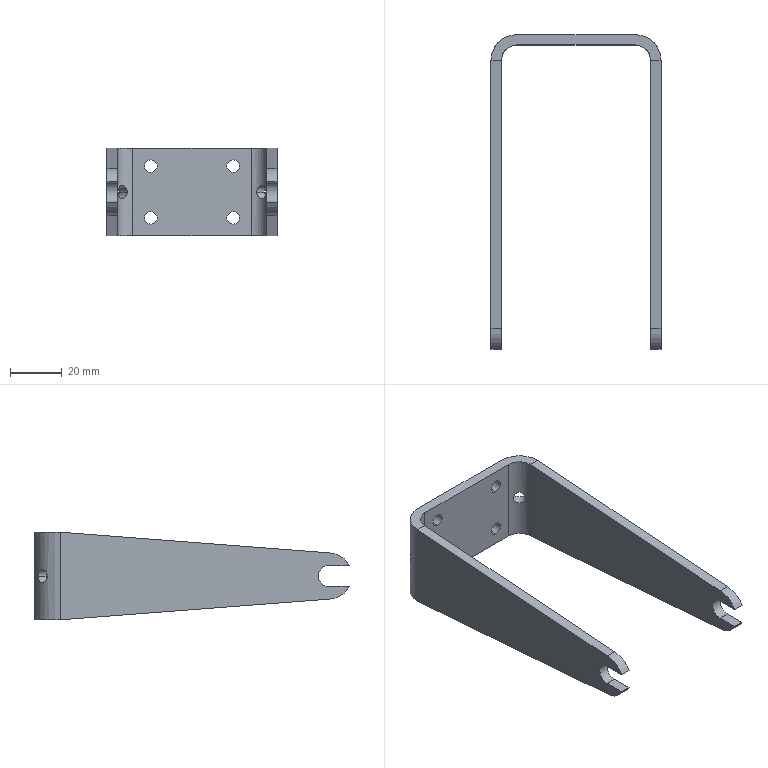Part | SolidWorks | features BaseBody 1 | 1 solid | 38 faces | box 66 x 122.062 x 34 mm | volume 31105 mm3 | cylinder 22 | plane 16 | commonest cylinder face diameters 4.9 x8 5 x4 18 x4 8 x2 12 x2 20 x2
STEP:
#1=CARTESIAN_POINT('',(25.089,57.125,0.));
#2=VERTEX_POINT('',#1);
#3=CARTESIAN_POINT('',(28.625,53.589,0.));
#4=VERTEX_POINT('',#3);
#5=CARTESIAN_POINT('',(25.089,57.125,0.));
#6=CARTESIAN_POINT('',(25.089,57.125,-0.1672));
#7=CARTESIAN_POINT('',(25.106,57.118,-0.3312));
#8=CARTESIAN_POINT('',(25.172,57.093,-0.6531));
#9=CARTESIAN_POINT('',(25.222,57.074,-0.8126));
#10=CARTESIAN_POINT('',(25.348,57.022,-1.114));
#11=CARTESIAN_POINT('',(25.424,56.989,-1.257));
#12=CARTESIAN_POINT('',(25.6,56.908,-1.527));
#13=CARTESIAN_POINT('',(25.698,56.86,-1.653));
#14=CARTESIAN_POINT('',(26.014,56.693,-1.995));
#15=CARTESIAN_POINT('',(26.258,56.548,-2.181));
#16=CARTESIAN_POINT('',(26.628,56.281,-2.369));
#17=CARTESIAN_POINT('',(26.755,56.182,-2.418));
#18=CARTESIAN_POINT('',(27.003,55.972,-2.483));
#19=CARTESIAN_POINT('',(27.123,55.862,-2.5));
#20=CARTESIAN_POINT('',(27.357,55.628,-2.5));
#21=CARTESIAN_POINT('',(27.471,55.505,-2.484));
#22=CARTESIAN_POINT('',(27.68,55.258,-2.419));
#23=CARTESIAN_POINT('',(27.778,55.133,-2.371));
#24=CARTESIAN_POINT('',(27.958,54.882,-2.244));
#25=CARTESIAN_POINT('',(28.039,54.761,-2.167));
#26=CARTESIAN_POINT('',(28.184,54.525,-1.986));
#27=CARTESIAN_POINT('',(28.248,54.41,-1.882));
#28=CARTESIAN_POINT('',(28.36,54.199,-1.654));
#29=CARTESIAN_POINT('',(28.408,54.101,-1.529));
#30=CARTESIAN_POINT('',(28.489,53.926,-1.26));
#31=CARTESIAN_POINT('',(28.522,53.849,-1.115));
#32=CARTESIAN_POINT('',(28.599,53.66,-0.6651));
#33=CARTESIAN_POINT('',(28.625,53.589,-0.3345));
#34=CARTESIAN_POINT('',(28.625,53.589,0.));
#35=B_SPLINE_CURVE_WITH_KNOTS('',3,(#5,#6,#7,#8,#9,#10,#11,#12,#13,#14,#15,#16,#17,#18,#19,#20,#21,#22,#23,#24,#25,#26,#27,#28,#29,#30,#31,#32,#33,#34),.UNSPECIFIED.,.F.,.F.,(4,2,2,2,2,2,2,2,2,2,2,2,2,2,4),(0.,0.0004939,0.0009879,0.001482,0.001976,0.002964,0.003458,0.003952,0.004446,0.004939,0.005433,0.005927,0.006421,0.006915,0.007903),.UNSPECIFIED.);
#36=EDGE_CURVE('',#2,#4,#35,.T.);
#37=ORIENTED_EDGE('',*,*,#36,.T.);
#38=CARTESIAN_POINT('',(31.614,56.579,0.));
#39=VERTEX_POINT('',#38);
#40=CARTESIAN_POINT('',(28.605,53.57,0.));
#41=DIRECTION('',(0.7071,0.7071,0.));
#42=VECTOR('',#41,1000.);
#43=LINE('',#40,#42);
#44=EDGE_CURVE('',#4,#39,#43,.T.);
#45=ORIENTED_EDGE('',*,*,#44,.T.);
#46=CARTESIAN_POINT('',(28.079,60.114,0.));
#47=VERTEX_POINT('',#46);
#48=CARTESIAN_POINT('',(31.614,56.579,0.));
#49=CARTESIAN_POINT('',(31.614,56.579,-0.1658));
#50=CARTESIAN_POINT('',(31.606,56.593,-0.3288));
#51=CARTESIAN_POINT('',(31.572,56.65,-0.6491));
#52=CARTESIAN_POINT('',(31.546,56.693,-0.8082));
#53=CARTESIAN_POINT('',(31.479,56.803,-1.111));
#54=CARTESIAN_POINT('',(31.437,56.869,-1.254));
#55=CARTESIAN_POINT('',(31.336,57.025,-1.525));
#56=CARTESIAN_POINT('',(31.276,57.114,-1.653));
#57=CARTESIAN_POINT('',(31.077,57.401,-1.997));
#58=CARTESIAN_POINT('',(30.909,57.627,-2.183));
#59=CARTESIAN_POINT('',(30.621,57.976,-2.371));
#60=CARTESIAN_POINT('',(30.518,58.096,-2.419));
#61=CARTESIAN_POINT('',(30.301,58.336,-2.484));
#62=CARTESIAN_POINT('',(30.188,58.454,-2.5));
#63=CARTESIAN_POINT('',(29.957,58.685,-2.5));
#64=CARTESIAN_POINT('',(29.836,58.8,-2.484));
#65=CARTESIAN_POINT('',(29.598,59.016,-2.42));
#66=CARTESIAN_POINT('',(29.48,59.118,-2.372));
#67=CARTESIAN_POINT('',(29.127,59.409,-2.184));
#68=CARTESIAN_POINT('',(28.904,59.575,-2.));
#69=CARTESIAN_POINT('',(28.614,59.776,-1.653));
#70=CARTESIAN_POINT('',(28.526,59.835,-1.527));
#71=CARTESIAN_POINT('',(28.371,59.936,-1.257));
#72=CARTESIAN_POINT('',(28.303,59.978,-1.111));
#73=CARTESIAN_POINT('',(28.193,60.046,-0.8094));
#74=CARTESIAN_POINT('',(28.151,60.071,-0.6536));
#75=CARTESIAN_POINT('',(28.094,60.106,-0.3318));
#76=CARTESIAN_POINT('',(28.079,60.114,-0.1658));
#77=CARTESIAN_POINT('',(28.079,60.114,0.));
#78=B_SPLINE_CURVE_WITH_KNOTS('',3,(#48,#49,#50,#51,#52,#53,#54,#55,#56,#57,#58,#59,#60,#61,#62,#63,#64,#65,#66,#67,#68,#69,#70,#71,#72,#73,#74,#75,#76,#77),.UNSPECIFIED.,.F.,.F.,(4,2,2,2,2,2,2,2,2,2,2,2,2,2,4),(0.,0.0004903,0.0009806,0.001471,0.001961,0.002942,0.003432,0.003922,0.004413,0.004903,0.005884,0.006374,0.006864,0.007355,0.007845),.UNSPECIFIED.);
#79=EDGE_CURVE('',#39,#47,#78,.T.);
#80=ORIENTED_EDGE('',*,*,#79,.T.);
#81=CARTESIAN_POINT('',(25.07,57.105,0.));
#82=DIRECTION('',(0.7071,0.7071,0.));
#83=VECTOR('',#82,1000.);
#84=LINE('',#81,#83);
#85=EDGE_CURVE('',#2,#47,#84,.T.);
#86=ORIENTED_EDGE('',*,*,#85,.F.);
#87=EDGE_LOOP('',(#37,#45,#80,#86));
#88=FACE_OUTER_BOUND('',#87,.T.);
#89=CARTESIAN_POINT('',(26.838,55.338,0.));
#90=DIRECTION('',(0.7071,0.7071,0.));
#91=DIRECTION('',(-0.7071,0.7071,0.));
#92=AXIS2_PLACEMENT_3D('',#89,#90,#91);
#93=CYLINDRICAL_SURFACE('',#92,2.5);
#94=ADVANCED_FACE('',(#88),#93,.F.);
#95=CARTESIAN_POINT('',(-16.,57.5,-7.55));
#96=VERTEX_POINT('',#95);
#97=CARTESIAN_POINT('',(-16.,57.5,-12.45));
#98=VERTEX_POINT('',#97);
#99=CARTESIAN_POINT('',(-16.,57.5,-10.));
#100=DIRECTION('',(0.,-1.,0.));
#101=DIRECTION('',(0.,0.,1.));
#102=AXIS2_PLACEMENT_3D('',#99,#100,#101);
#103=CIRCLE('',#102,2.45);
#104=EDGE_CURVE('',#96,#98,#103,.T.);
#105=ORIENTED_EDGE('',*,*,#104,.T.);
#106=CARTESIAN_POINT('',(-16.,61.5,-12.45));
#107=VERTEX_POINT('',#106);
#108=CARTESIAN_POINT('',(-16.,57.5,-12.45));
#109=DIRECTION('',(0.,1.,0.));
#110=VECTOR('',#109,1000.);
#111=LINE('',#108,#110);
#112=EDGE_CURVE('',#98,#107,#111,.T.);
#113=ORIENTED_EDGE('',*,*,#112,.T.);
#114=CARTESIAN_POINT('',(-16.,61.5,-7.55));
#115=VERTEX_POINT('',#114);
#116=CARTESIAN_POINT('',(-16.,61.5,-10.));
#117=DIRECTION('',(0.,1.,0.));
#118=DIRECTION('',(0.,0.,1.));
#119=AXIS2_PLACEMENT_3D('',#116,#117,#118);
#120=CIRCLE('',#119,2.45);
#121=EDGE_CURVE('',#107,#115,#120,.T.);
#122=ORIENTED_EDGE('',*,*,#121,.T.);
#123=CARTESIAN_POINT('',(-16.,57.5,-7.55));
#124=DIRECTION('',(0.,1.,0.));
#125=VECTOR('',#124,1000.);
#126=LINE('',#123,#125);
#127=EDGE_CURVE('',#96,#115,#126,.T.);
#128=ORIENTED_EDGE('',*,*,#127,.F.);
#129=EDGE_LOOP('',(#105,#113,#122,#128));
#130=FACE_OUTER_BOUND('',#129,.T.);
#131=CARTESIAN_POINT('',(-16.,57.5,-10.));
#132=DIRECTION('',(0.,1.,0.));
#133=DIRECTION('',(0.,0.,1.));
#134=AXIS2_PLACEMENT_3D('',#131,#132,#133);
#135=CYLINDRICAL_SURFACE('',#134,2.45);
#136=ADVANCED_FACE('',(#130),#135,.F.);
#137=CARTESIAN_POINT('',(16.,57.5,-7.55));
#138=VERTEX_POINT('',#137);
#139=CARTESIAN_POINT('',(16.,57.5,-12.45));
#140=VERTEX_POINT('',#139);
#141=CARTESIAN_POINT('',(16.,57.5,-10.));
#142=DIRECTION('',(0.,-1.,0.));
#143=DIRECTION('',(0.,0.,1.));
#144=AXIS2_PLACEMENT_3D('',#141,#142,#143);
#145=CIRCLE('',#144,2.45);
#146=EDGE_CURVE('',#138,#140,#145,.T.);
#147=ORIENTED_EDGE('',*,*,#146,.T.);
#148=CARTESIAN_POINT('',(16.,61.5,-12.45));
#149=VERTEX_POINT('',#148);
#150=CARTESIAN_POINT('',(16.,57.5,-12.45));
#151=DIRECTION('',(0.,1.,0.));
#152=VECTOR('',#151,1000.);
#153=LINE('',#150,#152);
#154=EDGE_CURVE('',#140,#149,#153,.T.);
#155=ORIENTED_EDGE('',*,*,#154,.T.);
#156=CARTESIAN_POINT('',(16.,61.5,-7.55));
#157=VERTEX_POINT('',#156);
#158=CARTESIAN_POINT('',(16.,61.5,-10.));
#159=DIRECTION('',(0.,1.,0.));
#160=DIRECTION('',(0.,0.,1.));
#161=AXIS2_PLACEMENT_3D('',#158,#159,#160);
#162=CIRCLE('',#161,2.45);
#163=EDGE_CURVE('',#149,#157,#162,.T.);
#164=ORIENTED_EDGE('',*,*,#163,.T.);
#165=CARTESIAN_POINT('',(16.,57.5,-7.55));
#166=DIRECTION('',(0.,1.,0.));
#167=VECTOR('',#166,1000.);
#168=LINE('',#165,#167);
#169=EDGE_CURVE('',#138,#157,#168,.T.);
#170=ORIENTED_EDGE('',*,*,#169,.F.);
#171=EDGE_LOOP('',(#147,#155,#164,#170));
#172=FACE_OUTER_BOUND('',#171,.T.);
#173=CARTESIAN_POINT('',(16.,57.5,-10.));
#174=DIRECTION('',(0.,1.,0.));
#175=DIRECTION('',(0.,0.,1.));
#176=AXIS2_PLACEMENT_3D('',#173,#174,#175);
#177=CYLINDRICAL_SURFACE('',#176,2.45);
#178=ADVANCED_FACE('',(#172),#177,.F.);
#179=CARTESIAN_POINT('',(-16.,57.5,12.45));
#180=VERTEX_POINT('',#179);
#181=CARTESIAN_POINT('',(-16.,57.5,7.55));
#182=VERTEX_POINT('',#181);
#183=CARTESIAN_POINT('',(-16.,57.5,10.));
#184=DIRECTION('',(0.,-1.,0.));
#185=DIRECTION('',(0.,0.,1.));
#186=AXIS2_PLACEMENT_3D('',#183,#184,#185);
#187=CIRCLE('',#186,2.45);
#188=EDGE_CURVE('',#180,#182,#187,.T.);
#189=ORIENTED_EDGE('',*,*,#188,.T.);
#190=CARTESIAN_POINT('',(-16.,61.5,7.55));
#191=VERTEX_POINT('',#190);
#192=CARTESIAN_POINT('',(-16.,57.5,7.55));
#193=DIRECTION('',(0.,1.,0.));
#194=VECTOR('',#193,1000.);
#195=LINE('',#192,#194);
#196=EDGE_CURVE('',#182,#191,#195,.T.);
#197=ORIENTED_EDGE('',*,*,#196,.T.);
#198=CARTESIAN_POINT('',(-16.,61.5,12.45));
#199=VERTEX_POINT('',#198);
#200=CARTESIAN_POINT('',(-16.,61.5,10.));
#201=DIRECTION('',(0.,1.,0.));
#202=DIRECTION('',(0.,0.,1.));
#203=AXIS2_PLACEMENT_3D('',#200,#201,#202);
#204=CIRCLE('',#203,2.45);
#205=EDGE_CURVE('',#191,#199,#204,.T.);
#206=ORIENTED_EDGE('',*,*,#205,.T.);
#207=CARTESIAN_POINT('',(-16.,57.5,12.45));
#208=DIRECTION('',(0.,1.,0.));
#209=VECTOR('',#208,1000.);
#210=LINE('',#207,#209);
#211=EDGE_CURVE('',#180,#199,#210,.T.);
#212=ORIENTED_EDGE('',*,*,#211,.F.);
#213=EDGE_LOOP('',(#189,#197,#206,#212));
#214=FACE_OUTER_BOUND('',#213,.T.);
#215=CARTESIAN_POINT('',(-16.,57.5,10.));
#216=DIRECTION('',(0.,1.,0.));
#217=DIRECTION('',(0.,0.,1.));
#218=AXIS2_PLACEMENT_3D('',#215,#216,#217);
#219=CYLINDRICAL_SURFACE('',#218,2.45);
#220=ADVANCED_FACE('',(#214),#219,.F.);
#221=CARTESIAN_POINT('',(16.,57.5,12.45));
#222=VERTEX_POINT('',#221);
#223=CARTESIAN_POINT('',(16.,57.5,7.55));
#224=VERTEX_POINT('',#223);
#225=CARTESIAN_POINT('',(16.,57.5,10.));
#226=DIRECTION('',(0.,-1.,0.));
#227=DIRECTION('',(0.,0.,1.));
#228=AXIS2_PLACEMENT_3D('',#225,#226,#227);
#229=CIRCLE('',#228,2.45);
#230=EDGE_CURVE('',#222,#224,#229,.T.);
#231=ORIENTED_EDGE('',*,*,#230,.T.);
#232=CARTESIAN_POINT('',(16.,61.5,7.55));
#233=VERTEX_POINT('',#232);
#234=CARTESIAN_POINT('',(16.,57.5,7.55));
#235=DIRECTION('',(0.,1.,0.));
#236=VECTOR('',#235,1000.);
#237=LINE('',#234,#236);
#238=EDGE_CURVE('',#224,#233,#237,.T.);
#239=ORIENTED_EDGE('',*,*,#238,.T.);
#240=CARTESIAN_POINT('',(16.,61.5,12.45));
#241=VERTEX_POINT('',#240);
#242=CARTESIAN_POINT('',(16.,61.5,10.));
#243=DIRECTION('',(0.,1.,0.));
#244=DIRECTION('',(0.,0.,1.));
#245=AXIS2_PLACEMENT_3D('',#242,#243,#244);
#246=CIRCLE('',#245,2.45);
#247=EDGE_CURVE('',#233,#241,#246,.T.);
#248=ORIENTED_EDGE('',*,*,#247,.T.);
#249=CARTESIAN_POINT('',(16.,57.5,12.45));
#250=DIRECTION('',(0.,1.,0.));
#251=VECTOR('',#250,1000.);
#252=LINE('',#249,#251);
#253=EDGE_CURVE('',#222,#241,#252,.T.);
#254=ORIENTED_EDGE('',*,*,#253,.F.);
#255=EDGE_LOOP('',(#231,#239,#248,#254));
#256=FACE_OUTER_BOUND('',#255,.T.);
#257=CARTESIAN_POINT('',(16.,57.5,10.));
#258=DIRECTION('',(0.,1.,0.));
#259=DIRECTION('',(0.,0.,1.));
#260=AXIS2_PLACEMENT_3D('',#257,#258,#259);
#261=CYLINDRICAL_SURFACE('',#260,2.45);
#262=ADVANCED_FACE('',(#256),#261,.F.);
#263=CARTESIAN_POINT('',(-25.089,57.125,0.));
#264=VERTEX_POINT('',#263);
#265=CARTESIAN_POINT('',(-28.625,53.589,0.));
#266=VERTEX_POINT('',#265);
#267=CARTESIAN_POINT('',(-25.089,57.125,0.));
#268=CARTESIAN_POINT('',(-25.089,57.125,-0.1672));
#269=CARTESIAN_POINT('',(-25.106,57.118,-0.3312));
#270=CARTESIAN_POINT('',(-25.172,57.093,-0.6531));
#271=CARTESIAN_POINT('',(-25.222,57.074,-0.8126));
#272=CARTESIAN_POINT('',(-25.348,57.022,-1.114));
#273=CARTESIAN_POINT('',(-25.424,56.989,-1.257));
#274=CARTESIAN_POINT('',(-25.6,56.908,-1.527));
#275=CARTESIAN_POINT('',(-25.698,56.86,-1.653));
#276=CARTESIAN_POINT('',(-26.014,56.693,-1.995));
#277=CARTESIAN_POINT('',(-26.258,56.548,-2.181));
#278=CARTESIAN_POINT('',(-26.628,56.281,-2.369));
#279=CARTESIAN_POINT('',(-26.755,56.182,-2.418));
#280=CARTESIAN_POINT('',(-27.003,55.972,-2.483));
#281=CARTESIAN_POINT('',(-27.123,55.862,-2.5));
#282=CARTESIAN_POINT('',(-27.357,55.628,-2.5));
#283=CARTESIAN_POINT('',(-27.471,55.505,-2.484));
#284=CARTESIAN_POINT('',(-27.68,55.258,-2.419));
#285=CARTESIAN_POINT('',(-27.778,55.133,-2.371));
#286=CARTESIAN_POINT('',(-27.958,54.882,-2.244));
#287=CARTESIAN_POINT('',(-28.039,54.761,-2.167));
#288=CARTESIAN_POINT('',(-28.184,54.525,-1.986));
#289=CARTESIAN_POINT('',(-28.248,54.41,-1.882));
#290=CARTESIAN_POINT('',(-28.36,54.199,-1.654));
#291=CARTESIAN_POINT('',(-28.408,54.101,-1.529));
#292=CARTESIAN_POINT('',(-28.489,53.926,-1.26));
#293=CARTESIAN_POINT('',(-28.522,53.849,-1.115));
#294=CARTESIAN_POINT('',(-28.599,53.66,-0.6651));
#295=CARTESIAN_POINT('',(-28.625,53.589,-0.3343));
#296=CARTESIAN_POINT('',(-28.625,53.589,0.));
#297=B_SPLINE_CURVE_WITH_KNOTS('',3,(#267,#268,#269,#270,#271,#272,#273,#274,#275,#276,#277,#278,#279,#280,#281,#282,#283,#284,#285,#286,#287,#288,#289,#290,#291,#292,#293,#294,#295,#296),.UNSPECIFIED.,.F.,.F.,(4,2,2,2,2,2,2,2,2,2,2,2,2,2,4),(0.007903,0.008397,0.008891,0.009385,0.009878,0.01087,0.01136,0.01185,0.01235,0.01284,0.01334,0.01383,0.01432,0.01482,0.0158),.UNSPECIFIED.);
#298=EDGE_CURVE('',#264,#266,#297,.T.);
#299=ORIENTED_EDGE('',*,*,#298,.F.);
#300=CARTESIAN_POINT('',(-28.079,60.114,0.));
#301=VERTEX_POINT('',#300);
#302=CARTESIAN_POINT('',(-25.07,57.105,0.));
#303=DIRECTION('',(-0.7071,0.7071,0.));
#304=VECTOR('',#303,1000.);
#305=LINE('',#302,#304);
#306=EDGE_CURVE('',#264,#301,#305,.T.);
#307=ORIENTED_EDGE('',*,*,#306,.T.);
#308=CARTESIAN_POINT('',(-31.614,56.579,0.));
#309=VERTEX_POINT('',#308);
#310=CARTESIAN_POINT('',(-28.079,60.114,0.));
#311=CARTESIAN_POINT('',(-28.079,60.114,-0.1658));
#312=CARTESIAN_POINT('',(-28.093,60.106,-0.3288));
#313=CARTESIAN_POINT('',(-28.15,60.072,-0.6491));
#314=CARTESIAN_POINT('',(-28.193,60.046,-0.8082));
#315=CARTESIAN_POINT('',(-28.303,59.979,-1.111));
#316=CARTESIAN_POINT('',(-28.369,59.937,-1.254));
#317=CARTESIAN_POINT('',(-28.525,59.836,-1.525));
#318=CARTESIAN_POINT('',(-28.614,59.776,-1.653));
#319=CARTESIAN_POINT('',(-28.901,59.577,-1.997));
#320=CARTESIAN_POINT('',(-29.127,59.409,-2.183));
#321=CARTESIAN_POINT('',(-29.476,59.121,-2.371));
#322=CARTESIAN_POINT('',(-29.596,59.018,-2.419));
#323=CARTESIAN_POINT('',(-29.836,58.801,-2.484));
#324=CARTESIAN_POINT('',(-29.954,58.688,-2.5));
#325=CARTESIAN_POINT('',(-30.185,58.457,-2.5));
#326=CARTESIAN_POINT('',(-30.3,58.336,-2.484));
#327=CARTESIAN_POINT('',(-30.516,58.098,-2.42));
#328=CARTESIAN_POINT('',(-30.618,57.98,-2.372));
#329=CARTESIAN_POINT('',(-30.909,57.627,-2.184));
#330=CARTESIAN_POINT('',(-31.075,57.404,-2.));
#331=CARTESIAN_POINT('',(-31.276,57.114,-1.653));
#332=CARTESIAN_POINT('',(-31.335,57.026,-1.527));
#333=CARTESIAN_POINT('',(-31.436,56.871,-1.257));
#334=CARTESIAN_POINT('',(-31.478,56.803,-1.111));
#335=CARTESIAN_POINT('',(-31.546,56.693,-0.8094));
#336=CARTESIAN_POINT('',(-31.571,56.651,-0.6536));
#337=CARTESIAN_POINT('',(-31.606,56.594,-0.3318));
#338=CARTESIAN_POINT('',(-31.614,56.579,-0.1658));
#339=CARTESIAN_POINT('',(-31.614,56.579,0.));
#340=B_SPLINE_CURVE_WITH_KNOTS('',3,(#310,#311,#312,#313,#314,#315,#316,#317,#318,#319,#320,#321,#322,#323,#324,#325,#326,#327,#328,#329,#330,#331,#332,#333,#334,#335,#336,#337,#338,#339),.UNSPECIFIED.,.F.,.F.,(4,2,2,2,2,2,2,2,2,2,2,2,2,2,4),(0.007845,0.008335,0.008825,0.009316,0.009806,0.01079,0.01128,0.01177,0.01226,0.01275,0.01373,0.01422,0.01471,0.0152,0.01569),.UNSPECIFIED.);
#341=EDGE_CURVE('',#301,#309,#340,.T.);
#342=ORIENTED_EDGE('',*,*,#341,.T.);
#343=CARTESIAN_POINT('',(-28.605,53.57,0.));
#344=DIRECTION('',(-0.7071,0.7071,0.));
#345=VECTOR('',#344,1000.);
#346=LINE('',#343,#345);
#347=EDGE_CURVE('',#266,#309,#346,.T.);
#348=ORIENTED_EDGE('',*,*,#347,.F.);
#349=EDGE_LOOP('',(#299,#307,#342,#348));
#350=FACE_OUTER_BOUND('',#349,.T.);
#351=CARTESIAN_POINT('',(-26.838,55.338,0.));
#352=DIRECTION('',(-0.7071,0.7071,0.));
#353=DIRECTION('',(-0.7071,-0.7071,0.));
#354=AXIS2_PLACEMENT_3D('',#351,#352,#353);
#355=CYLINDRICAL_SURFACE('',#354,2.5);
#356=ADVANCED_FACE('',(#350),#355,.F.);
#357=ORIENTED_EDGE('',*,*,#44,.F.);
#358=CARTESIAN_POINT('',(28.625,53.589,0.));
#359=CARTESIAN_POINT('',(28.625,53.589,0.1672));
#360=CARTESIAN_POINT('',(28.618,53.606,0.3312));
#361=CARTESIAN_POINT('',(28.593,53.672,0.6531));
#362=CARTESIAN_POINT('',(28.574,53.722,0.8126));
#363=CARTESIAN_POINT('',(28.522,53.848,1.114));
#364=CARTESIAN_POINT('',(28.489,53.924,1.257));
#365=CARTESIAN_POINT('',(28.408,54.1,1.527));
#366=CARTESIAN_POINT('',(28.36,54.198,1.653));
#367=CARTESIAN_POINT('',(28.193,54.514,1.995));
#368=CARTESIAN_POINT('',(28.048,54.758,2.181));
#369=CARTESIAN_POINT('',(27.781,55.128,2.369));
#370=CARTESIAN_POINT('',(27.682,55.255,2.418));
#371=CARTESIAN_POINT('',(27.472,55.503,2.483));
#372=CARTESIAN_POINT('',(27.362,55.623,2.5));
#373=CARTESIAN_POINT('',(27.128,55.857,2.5));
#374=CARTESIAN_POINT('',(27.005,55.971,2.484));
#375=CARTESIAN_POINT('',(26.758,56.18,2.419));
#376=CARTESIAN_POINT('',(26.633,56.278,2.371));
#377=CARTESIAN_POINT('',(26.382,56.458,2.244));
#378=CARTESIAN_POINT('',(26.261,56.539,2.167));
#379=CARTESIAN_POINT('',(26.025,56.684,1.986));
#380=CARTESIAN_POINT('',(25.91,56.748,1.882));
#381=CARTESIAN_POINT('',(25.699,56.86,1.654));
#382=CARTESIAN_POINT('',(25.601,56.908,1.529));
#383=CARTESIAN_POINT('',(25.426,56.989,1.26));
#384=CARTESIAN_POINT('',(25.349,57.022,1.115));
#385=CARTESIAN_POINT('',(25.16,57.099,0.6651));
#386=CARTESIAN_POINT('',(25.089,57.125,0.3343));
#387=CARTESIAN_POINT('',(25.089,57.125,0.));
#388=B_SPLINE_CURVE_WITH_KNOTS('',3,(#358,#359,#360,#361,#362,#363,#364,#365,#366,#367,#368,#369,#370,#371,#372,#373,#374,#375,#376,#377,#378,#379,#380,#381,#382,#383,#384,#385,#386,#387),.UNSPECIFIED.,.F.,.F.,(4,2,2,2,2,2,2,2,2,2,2,2,2,2,4),(0.007903,0.008397,0.008891,0.009385,0.009878,0.01087,0.01136,0.01185,0.01235,0.01284,0.01334,0.01383,0.01432,0.01482,0.0158),.UNSPECIFIED.);
#389=EDGE_CURVE('',#4,#2,#388,.T.);
#390=ORIENTED_EDGE('',*,*,#389,.T.);
#391=ORIENTED_EDGE('',*,*,#85,.T.);
#392=CARTESIAN_POINT('',(28.079,60.114,0.));
#393=CARTESIAN_POINT('',(28.079,60.114,0.1658));
#394=CARTESIAN_POINT('',(28.093,60.106,0.3288));
#395=CARTESIAN_POINT('',(28.15,60.072,0.6491));
#396=CARTESIAN_POINT('',(28.193,60.046,0.8082));
#397=CARTESIAN_POINT('',(28.303,59.979,1.111));
#398=CARTESIAN_POINT('',(28.369,59.937,1.254));
#399=CARTESIAN_POINT('',(28.525,59.836,1.525));
#400=CARTESIAN_POINT('',(28.614,59.776,1.653));
#401=CARTESIAN_POINT('',(28.901,59.577,1.997));
#402=CARTESIAN_POINT('',(29.127,59.409,2.183));
#403=CARTESIAN_POINT('',(29.476,59.121,2.371));
#404=CARTESIAN_POINT('',(29.596,59.018,2.419));
#405=CARTESIAN_POINT('',(29.836,58.801,2.484));
#406=CARTESIAN_POINT('',(29.954,58.688,2.5));
#407=CARTESIAN_POINT('',(30.185,58.457,2.5));
#408=CARTESIAN_POINT('',(30.3,58.336,2.484));
#409=CARTESIAN_POINT('',(30.516,58.098,2.42));
#410=CARTESIAN_POINT('',(30.618,57.98,2.372));
#411=CARTESIAN_POINT('',(30.909,57.627,2.184));
#412=CARTESIAN_POINT('',(31.075,57.404,2.));
#413=CARTESIAN_POINT('',(31.276,57.114,1.653));
#414=CARTESIAN_POINT('',(31.335,57.026,1.527));
#415=CARTESIAN_POINT('',(31.436,56.871,1.257));
#416=CARTESIAN_POINT('',(31.478,56.803,1.111));
#417=CARTESIAN_POINT('',(31.546,56.693,0.8094));
#418=CARTESIAN_POINT('',(31.571,56.651,0.6536));
#419=CARTESIAN_POINT('',(31.606,56.594,0.3318));
#420=CARTESIAN_POINT('',(31.614,56.579,0.1658));
#421=CARTESIAN_POINT('',(31.614,56.579,0.));
#422=B_SPLINE_CURVE_WITH_KNOTS('',3,(#392,#393,#394,#395,#396,#397,#398,#399,#400,#401,#402,#403,#404,#405,#406,#407,#408,#409,#410,#411,#412,#413,#414,#415,#416,#417,#418,#419,#420,#421),.UNSPECIFIED.,.F.,.F.,(4,2,2,2,2,2,2,2,2,2,2,2,2,2,4),(0.007845,0.008335,0.008825,0.009316,0.009806,0.01079,0.01128,0.01177,0.01226,0.01275,0.01373,0.01422,0.01471,0.0152,0.01569),.UNSPECIFIED.);
#423=EDGE_CURVE('',#47,#39,#422,.T.);
#424=ORIENTED_EDGE('',*,*,#423,.T.);
#425=EDGE_LOOP('',(#357,#390,#391,#424));
#426=FACE_OUTER_BOUND('',#425,.T.);
#427=CARTESIAN_POINT('',(26.838,55.338,0.));
#428=DIRECTION('',(0.7071,0.7071,0.));
#429=DIRECTION('',(-0.7071,0.7071,0.));
#430=AXIS2_PLACEMENT_3D('',#427,#428,#429);
#431=CYLINDRICAL_SURFACE('',#430,2.5);
#432=ADVANCED_FACE('',(#426),#431,.F.);
#433=CARTESIAN_POINT('',(23.,61.5,17.));
#434=VERTEX_POINT('',#433);
#435=CARTESIAN_POINT('',(23.,61.5,-17.));
#436=VERTEX_POINT('',#435);
#437=CARTESIAN_POINT('',(23.,61.5,0.));
#438=DIRECTION('',(0.,0.,-1.));
#439=VECTOR('',#438,1000.);
#440=LINE('',#437,#439);
#441=EDGE_CURVE('',#434,#436,#440,.T.);
#442=ORIENTED_EDGE('',*,*,#441,.F.);
#443=CARTESIAN_POINT('',(33.,51.5,17.));
#444=VERTEX_POINT('',#443);
#445=CARTESIAN_POINT('',(23.,51.5,17.));
#446=DIRECTION('',(0.,0.,1.));
#447=DIRECTION('',(-1.,0.,0.));
#448=AXIS2_PLACEMENT_3D('',#445,#446,#447);
#449=CIRCLE('',#448,10.);
#450=EDGE_CURVE('',#444,#434,#449,.T.);
#451=ORIENTED_EDGE('',*,*,#450,.F.);
#452=CARTESIAN_POINT('',(33.,51.5,-17.));
#453=VERTEX_POINT('',#452);
#454=CARTESIAN_POINT('',(33.,51.5,0.));
#455=DIRECTION('',(0.,0.,1.));
#456=VECTOR('',#455,1000.);
#457=LINE('',#454,#456);
#458=EDGE_CURVE('',#453,#444,#457,.T.);
#459=ORIENTED_EDGE('',*,*,#458,.F.);
#460=CARTESIAN_POINT('',(23.,51.5,-17.));
#461=DIRECTION('',(0.,0.,-1.));
#462=DIRECTION('',(-1.,0.,0.));
#463=AXIS2_PLACEMENT_3D('',#460,#461,#462);
#464=CIRCLE('',#463,10.);
#465=EDGE_CURVE('',#436,#453,#464,.T.);
#466=ORIENTED_EDGE('',*,*,#465,.F.);
#467=EDGE_LOOP('',(#442,#451,#459,#466));
#468=FACE_OUTER_BOUND('',#467,.T.);
#469=ORIENTED_EDGE('',*,*,#423,.F.);
#470=ORIENTED_EDGE('',*,*,#79,.F.);
#471=EDGE_LOOP('',(#469,#470));
#472=FACE_BOUND('',#471,.T.);
#473=CARTESIAN_POINT('',(23.,51.5,17.));
#474=DIRECTION('',(0.,0.,-1.));
#475=DIRECTION('',(-1.,0.,0.));
#476=AXIS2_PLACEMENT_3D('',#473,#474,#475);
#477=CYLINDRICAL_SURFACE('',#476,10.);
#478=ADVANCED_FACE('',(#468,#472),#477,.T.);
#479=CARTESIAN_POINT('',(29.,51.5,17.));
#480=VERTEX_POINT('',#479);
#481=CARTESIAN_POINT('',(23.,57.5,17.));
#482=VERTEX_POINT('',#481);
#483=CARTESIAN_POINT('',(23.,51.5,17.));
#484=DIRECTION('',(0.,0.,1.));
#485=DIRECTION('',(-1.,0.,0.));
#486=AXIS2_PLACEMENT_3D('',#483,#484,#485);
#487=CIRCLE('',#486,6.);
#488=EDGE_CURVE('',#480,#482,#487,.T.);
#489=ORIENTED_EDGE('',*,*,#488,.T.);
#490=CARTESIAN_POINT('',(23.,57.5,-17.));
#491=VERTEX_POINT('',#490);
#492=CARTESIAN_POINT('',(23.,57.5,0.));
#493=DIRECTION('',(0.,0.,-1.));
#494=VECTOR('',#493,1000.);
#495=LINE('',#492,#494);
#496=EDGE_CURVE('',#482,#491,#495,.T.);
#497=ORIENTED_EDGE('',*,*,#496,.T.);
#498=CARTESIAN_POINT('',(29.,51.5,-17.));
#499=VERTEX_POINT('',#498);
#500=CARTESIAN_POINT('',(23.,51.5,-17.));
#501=DIRECTION('',(0.,0.,-1.));
#502=DIRECTION('',(-1.,0.,0.));
#503=AXIS2_PLACEMENT_3D('',#500,#501,#502);
#504=CIRCLE('',#503,6.);
#505=EDGE_CURVE('',#491,#499,#504,.T.);
#506=ORIENTED_EDGE('',*,*,#505,.T.);
#507=CARTESIAN_POINT('',(29.,51.5,0.));
#508=DIRECTION('',(0.,0.,1.));
#509=VECTOR('',#508,1000.);
#510=LINE('',#507,#509);
#511=EDGE_CURVE('',#499,#480,#510,.T.);
#512=ORIENTED_EDGE('',*,*,#511,.T.);
#513=EDGE_LOOP('',(#489,#497,#506,#512));
#514=FACE_OUTER_BOUND('',#513,.T.);
#515=ORIENTED_EDGE('',*,*,#36,.F.);
#516=ORIENTED_EDGE('',*,*,#389,.F.);
#517=EDGE_LOOP('',(#515,#516));
#518=FACE_BOUND('',#517,.T.);
#519=CARTESIAN_POINT('',(23.,51.5,17.));
#520=DIRECTION('',(0.,0.,-1.));
#521=DIRECTION('',(-1.,0.,0.));
#522=AXIS2_PLACEMENT_3D('',#519,#520,#521);
#523=CYLINDRICAL_SURFACE('',#522,6.);
#524=ADVANCED_FACE('',(#514,#518),#523,.F.);
#525=CARTESIAN_POINT('',(0.,51.5,-17.));
#526=DIRECTION('',(1.,0.,0.));
#527=VECTOR('',#526,1000.);
#528=LINE('',#525,#527);
#529=EDGE_CURVE('',#499,#453,#528,.T.);
#530=ORIENTED_EDGE('',*,*,#529,.F.);
#531=ORIENTED_EDGE('',*,*,#505,.F.);
#532=CARTESIAN_POINT('',(-23.,57.5,-17.));
#533=VERTEX_POINT('',#532);
#534=CARTESIAN_POINT('',(0.,57.5,-17.));
#535=DIRECTION('',(1.,0.,0.));
#536=VECTOR('',#535,1000.);
#537=LINE('',#534,#536);
#538=EDGE_CURVE('',#533,#491,#537,.T.);
#539=ORIENTED_EDGE('',*,*,#538,.F.);
#540=CARTESIAN_POINT('',(-29.,51.5,-17.));
#541=VERTEX_POINT('',#540);
#542=CARTESIAN_POINT('',(-23.,51.5,-17.));
#543=DIRECTION('',(0.,0.,-1.));
#544=DIRECTION('',(-1.,0.,0.));
#545=AXIS2_PLACEMENT_3D('',#542,#543,#544);
#546=CIRCLE('',#545,6.);
#547=EDGE_CURVE('',#541,#533,#546,.T.);
#548=ORIENTED_EDGE('',*,*,#547,.F.);
#549=CARTESIAN_POINT('',(-33.,51.5,-17.));
#550=VERTEX_POINT('',#549);
#551=CARTESIAN_POINT('',(0.,51.5,-17.));
#552=DIRECTION('',(1.,0.,0.));
#553=VECTOR('',#552,1000.);
#554=LINE('',#551,#553);
#555=EDGE_CURVE('',#550,#541,#554,.T.);
#556=ORIENTED_EDGE('',*,*,#555,.F.);
#557=CARTESIAN_POINT('',(-23.,61.5,-17.));
#558=VERTEX_POINT('',#557);
#559=CARTESIAN_POINT('',(-23.,51.5,-17.));
#560=DIRECTION('',(0.,0.,1.));
#561=DIRECTION('',(-1.,0.,0.));
#562=AXIS2_PLACEMENT_3D('',#559,#560,#561);
#563=CIRCLE('',#562,10.);
#564=EDGE_CURVE('',#558,#550,#563,.T.);
#565=ORIENTED_EDGE('',*,*,#564,.F.);
#566=CARTESIAN_POINT('',(0.,61.5,-17.));
#567=DIRECTION('',(-1.,0.,0.));
#568=VECTOR('',#567,1000.);
#569=LINE('',#566,#568);
#570=EDGE_CURVE('',#436,#558,#569,.T.);
#571=ORIENTED_EDGE('',*,*,#570,.F.);
#572=ORIENTED_EDGE('',*,*,#465,.T.);
#573=EDGE_LOOP('',(#530,#531,#539,#548,#556,#565,#571,#572));
#574=FACE_OUTER_BOUND('',#573,.T.);
#575=CARTESIAN_POINT('',(-33.396,51.5,-17.));
#576=DIRECTION('',(0.,0.,1.));
#577=DIRECTION('',(1.,0.,0.));
#578=AXIS2_PLACEMENT_3D('',#575,#576,#577);
#579=PLANE('',#578);
#580=ADVANCED_FACE('',(#574),#579,.F.);
#581=CARTESIAN_POINT('',(-16.,61.5,-10.));
#582=DIRECTION('',(0.,1.,0.));
#583=DIRECTION('',(0.,0.,1.));
#584=AXIS2_PLACEMENT_3D('',#581,#582,#583);
#585=CIRCLE('',#584,2.45);
#586=EDGE_CURVE('',#115,#107,#585,.T.);
#587=ORIENTED_EDGE('',*,*,#586,.F.);
#588=ORIENTED_EDGE('',*,*,#121,.F.);
#589=EDGE_LOOP('',(#587,#588));
#590=FACE_BOUND('',#589,.T.);
#591=CARTESIAN_POINT('',(16.,61.5,-10.));
#592=DIRECTION('',(0.,1.,0.));
#593=DIRECTION('',(0.,0.,1.));
#594=AXIS2_PLACEMENT_3D('',#591,#592,#593);
#595=CIRCLE('',#594,2.45);
#596=EDGE_CURVE('',#157,#149,#595,.T.);
#597=ORIENTED_EDGE('',*,*,#596,.F.);
#598=ORIENTED_EDGE('',*,*,#163,.F.);
#599=EDGE_LOOP('',(#597,#598));
#600=FACE_BOUND('',#599,.T.);
#601=CARTESIAN_POINT('',(-16.,61.5,10.));
#602=DIRECTION('',(0.,1.,0.));
#603=DIRECTION('',(0.,0.,1.));
#604=AXIS2_PLACEMENT_3D('',#601,#602,#603);
#605=CIRCLE('',#604,2.45);
#606=EDGE_CURVE('',#199,#191,#605,.T.);
#607=ORIENTED_EDGE('',*,*,#606,.F.);
#608=ORIENTED_EDGE('',*,*,#205,.F.);
#609=EDGE_LOOP('',(#607,#608));
#610=FACE_BOUND('',#609,.T.);
#611=CARTESIAN_POINT('',(16.,61.5,10.));
#612=DIRECTION('',(0.,1.,0.));
#613=DIRECTION('',(0.,0.,1.));
#614=AXIS2_PLACEMENT_3D('',#611,#612,#613);
#615=CIRCLE('',#614,2.45);
#616=EDGE_CURVE('',#241,#233,#615,.T.);
#617=ORIENTED_EDGE('',*,*,#616,.F.);
#618=ORIENTED_EDGE('',*,*,#247,.F.);
#619=EDGE_LOOP('',(#617,#618));
#620=FACE_BOUND('',#619,.T.);
#621=CARTESIAN_POINT('',(-23.,61.5,17.));
#622=VERTEX_POINT('',#621);
#623=CARTESIAN_POINT('',(-23.,61.5,0.));
#624=DIRECTION('',(0.,0.,-1.));
#625=VECTOR('',#624,1000.);
#626=LINE('',#623,#625);
#627=EDGE_CURVE('',#622,#558,#626,.T.);
#628=ORIENTED_EDGE('',*,*,#627,.F.);
#629=CARTESIAN_POINT('',(0.,61.5,17.));
#630=DIRECTION('',(-1.,0.,0.));
#631=VECTOR('',#630,1000.);
#632=LINE('',#629,#631);
#633=EDGE_CURVE('',#434,#622,#632,.T.);
#634=ORIENTED_EDGE('',*,*,#633,.F.);
#635=ORIENTED_EDGE('',*,*,#441,.T.);
#636=ORIENTED_EDGE('',*,*,#570,.T.);
#637=EDGE_LOOP('',(#628,#634,#635,#636));
#638=FACE_OUTER_BOUND('',#637,.T.);
#639=CARTESIAN_POINT('',(-23.,61.5,-17.));
#640=DIRECTION('',(0.,-1.,0.));
#641=DIRECTION('',(1.,0.,0.));
#642=AXIS2_PLACEMENT_3D('',#639,#640,#641);
#643=PLANE('',#642);
#644=ADVANCED_FACE('',(#590,#600,#610,#620,#638),#643,.F.);
#645=CARTESIAN_POINT('',(-23.,57.5,17.));
#646=VERTEX_POINT('',#645);
#647=CARTESIAN_POINT('',(0.,57.5,17.));
#648=DIRECTION('',(1.,0.,0.));
#649=VECTOR('',#648,1000.);
#650=LINE('',#647,#649);
#651=EDGE_CURVE('',#646,#482,#650,.T.);
#652=ORIENTED_EDGE('',*,*,#651,.T.);
#653=ORIENTED_EDGE('',*,*,#488,.F.);
#654=CARTESIAN_POINT('',(0.,51.5,17.));
#655=DIRECTION('',(1.,0.,0.));
#656=VECTOR('',#655,1000.);
#657=LINE('',#654,#656);
#658=EDGE_CURVE('',#480,#444,#657,.T.);
#659=ORIENTED_EDGE('',*,*,#658,.T.);
#660=ORIENTED_EDGE('',*,*,#450,.T.);
#661=ORIENTED_EDGE('',*,*,#633,.T.);
#662=CARTESIAN_POINT('',(-33.,51.5,17.));
#663=VERTEX_POINT('',#662);
#664=CARTESIAN_POINT('',(-23.,51.5,17.));
#665=DIRECTION('',(0.,0.,1.));
#666=DIRECTION('',(-1.,0.,0.));
#667=AXIS2_PLACEMENT_3D('',#664,#665,#666);
#668=CIRCLE('',#667,10.);
#669=EDGE_CURVE('',#622,#663,#668,.T.);
#670=ORIENTED_EDGE('',*,*,#669,.T.);
#671=CARTESIAN_POINT('',(-29.,51.5,17.));
#672=VERTEX_POINT('',#671);
#673=CARTESIAN_POINT('',(0.,51.5,17.));
#674=DIRECTION('',(1.,0.,0.));
#675=VECTOR('',#674,1000.);
#676=LINE('',#673,#675);
#677=EDGE_CURVE('',#663,#672,#676,.T.);
#678=ORIENTED_EDGE('',*,*,#677,.T.);
#679=CARTESIAN_POINT('',(-23.,51.5,17.));
#680=DIRECTION('',(0.,0.,-1.));
#681=DIRECTION('',(-1.,0.,0.));
#682=AXIS2_PLACEMENT_3D('',#679,#680,#681);
#683=CIRCLE('',#682,6.);
#684=EDGE_CURVE('',#672,#646,#683,.T.);
#685=ORIENTED_EDGE('',*,*,#684,.T.);
#686=EDGE_LOOP('',(#652,#653,#659,#660,#661,#670,#678,#685));
#687=FACE_OUTER_BOUND('',#686,.T.);
#688=CARTESIAN_POINT('',(-33.396,51.5,17.));
#689=DIRECTION('',(0.,0.,1.));
#690=DIRECTION('',(1.,0.,0.));
#691=AXIS2_PLACEMENT_3D('',#688,#689,#690);
#692=PLANE('',#691);
#693=ADVANCED_FACE('',(#687),#692,.T.);
#694=CARTESIAN_POINT('',(33.,-52.5,9.));
#695=VERTEX_POINT('',#694);
#696=CARTESIAN_POINT('',(33.,-52.5,9.));
#697=DIRECTION('',(0.,0.9971,0.0767));
#698=VECTOR('',#697,1000.);
#699=LINE('',#696,#698);
#700=EDGE_CURVE('',#695,#444,#699,.T.);
#701=ORIENTED_EDGE('',*,*,#700,.F.);
#702=CARTESIAN_POINT('',(33.,-60.562,4.));
#703=VERTEX_POINT('',#702);
#704=CARTESIAN_POINT('',(33.,-52.5,0.));
#705=DIRECTION('',(-1.,0.,0.));
#706=DIRECTION('',(0.,0.,-1.));
#707=AXIS2_PLACEMENT_3D('',#704,#705,#706);
#708=CIRCLE('',#707,9.);
#709=EDGE_CURVE('',#703,#695,#708,.T.);
#710=ORIENTED_EDGE('',*,*,#709,.F.);
#711=CARTESIAN_POINT('',(33.,-52.5,4.));
#712=VERTEX_POINT('',#711);
#713=CARTESIAN_POINT('',(33.,-4.867,4.));
#714=DIRECTION('',(0.,-1.,0.));
#715=VECTOR('',#714,1000.);
#716=LINE('',#713,#715);
#717=EDGE_CURVE('',#712,#703,#716,.T.);
#718=ORIENTED_EDGE('',*,*,#717,.F.);
#719=CARTESIAN_POINT('',(33.,-52.5,-4.));
#720=VERTEX_POINT('',#719);
#721=CARTESIAN_POINT('',(33.,-52.5,0.));
#722=DIRECTION('',(1.,0.,0.));
#723=DIRECTION('',(0.,0.,-1.));
#724=AXIS2_PLACEMENT_3D('',#721,#722,#723);
#725=CIRCLE('',#724,4.);
#726=EDGE_CURVE('',#720,#712,#725,.T.);
#727=ORIENTED_EDGE('',*,*,#726,.F.);
#728=CARTESIAN_POINT('',(33.,-60.562,-4.));
#729=VERTEX_POINT('',#728);
#730=CARTESIAN_POINT('',(33.,-4.867,-4.));
#731=DIRECTION('',(0.,1.,0.));
#732=VECTOR('',#731,1000.);
#733=LINE('',#730,#732);
#734=EDGE_CURVE('',#729,#720,#733,.T.);
#735=ORIENTED_EDGE('',*,*,#734,.F.);
#736=CARTESIAN_POINT('',(33.,-52.5,-9.));
#737=VERTEX_POINT('',#736);
#738=CARTESIAN_POINT('',(33.,-52.5,0.));
#739=DIRECTION('',(-1.,0.,0.));
#740=DIRECTION('',(0.,0.,-1.));
#741=AXIS2_PLACEMENT_3D('',#738,#739,#740);
#742=CIRCLE('',#741,9.);
#743=EDGE_CURVE('',#737,#729,#742,.T.);
#744=ORIENTED_EDGE('',*,*,#743,.F.);
#745=CARTESIAN_POINT('',(33.,51.5,-17.));
#746=DIRECTION('',(0.,-0.9971,0.0767));
#747=VECTOR('',#746,1000.);
#748=LINE('',#745,#747);
#749=EDGE_CURVE('',#453,#737,#748,.T.);
#750=ORIENTED_EDGE('',*,*,#749,.F.);
#751=ORIENTED_EDGE('',*,*,#458,.T.);
#752=EDGE_LOOP('',(#701,#710,#718,#727,#735,#744,#750,#751));
#753=FACE_OUTER_BOUND('',#752,.T.);
#754=CARTESIAN_POINT('',(33.,51.5,-17.204));
#755=DIRECTION('',(-1.,0.,0.));
#756=DIRECTION('',(0.,-1.,0.));
#757=AXIS2_PLACEMENT_3D('',#754,#755,#756);
#758=PLANE('',#757);
#759=ADVANCED_FACE('',(#753),#758,.F.);
#760=ORIENTED_EDGE('',*,*,#104,.F.);
#761=CARTESIAN_POINT('',(-16.,57.5,-10.));
#762=DIRECTION('',(0.,-1.,0.));
#763=DIRECTION('',(0.,0.,1.));
#764=AXIS2_PLACEMENT_3D('',#761,#762,#763);
#765=CIRCLE('',#764,2.45);
#766=EDGE_CURVE('',#98,#96,#765,.T.);
#767=ORIENTED_EDGE('',*,*,#766,.F.);
#768=EDGE_LOOP('',(#760,#767));
#769=FACE_BOUND('',#768,.T.);
#770=ORIENTED_EDGE('',*,*,#146,.F.);
#771=CARTESIAN_POINT('',(16.,57.5,-10.));
#772=DIRECTION('',(0.,-1.,0.));
#773=DIRECTION('',(0.,0.,1.));
#774=AXIS2_PLACEMENT_3D('',#771,#772,#773);
#775=CIRCLE('',#774,2.45);
#776=EDGE_CURVE('',#140,#138,#775,.T.);
#777=ORIENTED_EDGE('',*,*,#776,.F.);
#778=EDGE_LOOP('',(#770,#777));
#779=FACE_BOUND('',#778,.T.);
#780=ORIENTED_EDGE('',*,*,#188,.F.);
#781=CARTESIAN_POINT('',(-16.,57.5,10.));
#782=DIRECTION('',(0.,-1.,0.));
#783=DIRECTION('',(0.,0.,1.));
#784=AXIS2_PLACEMENT_3D('',#781,#782,#783);
#785=CIRCLE('',#784,2.45);
#786=EDGE_CURVE('',#182,#180,#785,.T.);
#787=ORIENTED_EDGE('',*,*,#786,.F.);
#788=EDGE_LOOP('',(#780,#787));
#789=FACE_BOUND('',#788,.T.);
#790=ORIENTED_EDGE('',*,*,#230,.F.);
#791=CARTESIAN_POINT('',(16.,57.5,10.));
#792=DIRECTION('',(0.,-1.,0.));
#793=DIRECTION('',(0.,0.,1.));
#794=AXIS2_PLACEMENT_3D('',#791,#792,#793);
#795=CIRCLE('',#794,2.45);
#796=EDGE_CURVE('',#224,#222,#795,.T.);
#797=ORIENTED_EDGE('',*,*,#796,.F.);
#798=EDGE_LOOP('',(#790,#797));
#799=FACE_BOUND('',#798,.T.);
#800=ORIENTED_EDGE('',*,*,#496,.F.);
#801=ORIENTED_EDGE('',*,*,#651,.F.);
#802=CARTESIAN_POINT('',(-23.,57.5,0.));
#803=DIRECTION('',(0.,0.,1.));
#804=VECTOR('',#803,1000.);
#805=LINE('',#802,#804);
#806=EDGE_CURVE('',#533,#646,#805,.T.);
#807=ORIENTED_EDGE('',*,*,#806,.F.);
#808=ORIENTED_EDGE('',*,*,#538,.T.);
#809=EDGE_LOOP('',(#800,#801,#807,#808));
#810=FACE_OUTER_BOUND('',#809,.T.);
#811=CARTESIAN_POINT('',(23.,57.5,-17.));
#812=DIRECTION('',(0.,1.,0.));
#813=DIRECTION('',(-1.,0.,0.));
#814=AXIS2_PLACEMENT_3D('',#811,#812,#813);
#815=PLANE('',#814);
#816=ADVANCED_FACE('',(#769,#779,#789,#799,#810),#815,.F.);
#817=CARTESIAN_POINT('',(29.,-52.5,9.));
#818=VERTEX_POINT('',#817);
#819=CARTESIAN_POINT('',(29.,-52.5,9.));
#820=DIRECTION('',(0.,-0.9971,-0.0767));
#821=VECTOR('',#820,1000.);
#822=LINE('',#819,#821);
#823=EDGE_CURVE('',#480,#818,#822,.T.);
#824=ORIENTED_EDGE('',*,*,#823,.F.);
#825=ORIENTED_EDGE('',*,*,#511,.F.);
#826=CARTESIAN_POINT('',(29.,-52.5,-9.));
#827=VERTEX_POINT('',#826);
#828=CARTESIAN_POINT('',(29.,51.5,-17.));
#829=DIRECTION('',(0.,0.9971,-0.0767));
#830=VECTOR('',#829,1000.);
#831=LINE('',#828,#830);
#832=EDGE_CURVE('',#827,#499,#831,.T.);
#833=ORIENTED_EDGE('',*,*,#832,.F.);
#834=CARTESIAN_POINT('',(29.,-60.562,-4.));
#835=VERTEX_POINT('',#834);
#836=CARTESIAN_POINT('',(29.,-52.5,0.));
#837=DIRECTION('',(1.,0.,0.));
#838=DIRECTION('',(0.,0.,-1.));
#839=AXIS2_PLACEMENT_3D('',#836,#837,#838);
#840=CIRCLE('',#839,9.);
#841=EDGE_CURVE('',#835,#827,#840,.T.);
#842=ORIENTED_EDGE('',*,*,#841,.F.);
#843=CARTESIAN_POINT('',(29.,-52.5,-4.));
#844=VERTEX_POINT('',#843);
#845=CARTESIAN_POINT('',(29.,-4.867,-4.));
#846=DIRECTION('',(0.,-1.,0.));
#847=VECTOR('',#846,1000.);
#848=LINE('',#845,#847);
#849=EDGE_CURVE('',#844,#835,#848,.T.);
#850=ORIENTED_EDGE('',*,*,#849,.F.);
#851=CARTESIAN_POINT('',(29.,-52.5,4.));
#852=VERTEX_POINT('',#851);
#853=CARTESIAN_POINT('',(29.,-52.5,0.));
#854=DIRECTION('',(-1.,0.,0.));
#855=DIRECTION('',(0.,0.,-1.));
#856=AXIS2_PLACEMENT_3D('',#853,#854,#855);
#857=CIRCLE('',#856,4.);
#858=EDGE_CURVE('',#852,#844,#857,.T.);
#859=ORIENTED_EDGE('',*,*,#858,.F.);
#860=CARTESIAN_POINT('',(29.,-60.562,4.));
#861=VERTEX_POINT('',#860);
#862=CARTESIAN_POINT('',(29.,-4.867,4.));
#863=DIRECTION('',(0.,1.,0.));
#864=VECTOR('',#863,1000.);
#865=LINE('',#862,#864);
#866=EDGE_CURVE('',#861,#852,#865,.T.);
#867=ORIENTED_EDGE('',*,*,#866,.F.);
#868=CARTESIAN_POINT('',(29.,-52.5,0.));
#869=DIRECTION('',(1.,0.,0.));
#870=DIRECTION('',(0.,0.,-1.));
#871=AXIS2_PLACEMENT_3D('',#868,#869,#870);
#872=CIRCLE('',#871,9.);
#873=EDGE_CURVE('',#818,#861,#872,.T.);
#874=ORIENTED_EDGE('',*,*,#873,.F.);
#875=EDGE_LOOP('',(#824,#825,#833,#842,#850,#859,#867,#874));
#876=FACE_OUTER_BOUND('',#875,.T.);
#877=CARTESIAN_POINT('',(29.,-61.235,17.204));
#878=DIRECTION('',(1.,0.,0.));
#879=DIRECTION('',(0.,0.,-1.));
#880=AXIS2_PLACEMENT_3D('',#877,#878,#879);
#881=PLANE('',#880);
#882=ADVANCED_FACE('',(#876),#881,.F.);
#883=ORIENTED_EDGE('',*,*,#749,.T.);
#884=CARTESIAN_POINT('',(31.,-52.5,-9.));
#885=DIRECTION('',(1.,0.,0.));
#886=VECTOR('',#885,1000.);
#887=LINE('',#884,#886);
#888=EDGE_CURVE('',#827,#737,#887,.T.);
#889=ORIENTED_EDGE('',*,*,#888,.F.);
#890=ORIENTED_EDGE('',*,*,#832,.T.);
#891=ORIENTED_EDGE('',*,*,#529,.T.);
#892=EDGE_LOOP('',(#883,#889,#890,#891));
#893=FACE_OUTER_BOUND('',#892,.T.);
#894=CARTESIAN_POINT('',(29.,51.5,-17.));
#895=DIRECTION('',(0.,0.0767,0.9971));
#896=DIRECTION('',(0.,-0.9971,0.0767));
#897=AXIS2_PLACEMENT_3D('',#894,#895,#896);
#898=PLANE('',#897);
#899=ADVANCED_FACE('',(#893),#898,.F.);
#900=ORIENTED_EDGE('',*,*,#684,.F.);
#901=CARTESIAN_POINT('',(-29.,51.5,0.));
#902=DIRECTION('',(0.,0.,-1.));
#903=VECTOR('',#902,1000.);
#904=LINE('',#901,#903);
#905=EDGE_CURVE('',#672,#541,#904,.T.);
#906=ORIENTED_EDGE('',*,*,#905,.T.);
#907=ORIENTED_EDGE('',*,*,#547,.T.);
#908=ORIENTED_EDGE('',*,*,#806,.T.);
#909=EDGE_LOOP('',(#900,#906,#907,#908));
#910=FACE_OUTER_BOUND('',#909,.T.);
#911=CARTESIAN_POINT('',(-28.625,53.589,0.));
#912=CARTESIAN_POINT('',(-28.625,53.589,0.1672));
#913=CARTESIAN_POINT('',(-28.618,53.606,0.3312));
#914=CARTESIAN_POINT('',(-28.593,53.672,0.6531));
#915=CARTESIAN_POINT('',(-28.574,53.722,0.8126));
#916=CARTESIAN_POINT('',(-28.522,53.848,1.114));
#917=CARTESIAN_POINT('',(-28.489,53.924,1.257));
#918=CARTESIAN_POINT('',(-28.408,54.1,1.527));
#919=CARTESIAN_POINT('',(-28.36,54.198,1.653));
#920=CARTESIAN_POINT('',(-28.193,54.514,1.995));
#921=CARTESIAN_POINT('',(-28.048,54.758,2.181));
#922=CARTESIAN_POINT('',(-27.781,55.128,2.369));
#923=CARTESIAN_POINT('',(-27.682,55.255,2.418));
#924=CARTESIAN_POINT('',(-27.472,55.503,2.483));
#925=CARTESIAN_POINT('',(-27.362,55.623,2.5));
#926=CARTESIAN_POINT('',(-27.128,55.857,2.5));
#927=CARTESIAN_POINT('',(-27.005,55.971,2.484));
#928=CARTESIAN_POINT('',(-26.758,56.18,2.419));
#929=CARTESIAN_POINT('',(-26.633,56.278,2.371));
#930=CARTESIAN_POINT('',(-26.382,56.458,2.244));
#931=CARTESIAN_POINT('',(-26.261,56.539,2.167));
#932=CARTESIAN_POINT('',(-26.025,56.684,1.986));
#933=CARTESIAN_POINT('',(-25.91,56.748,1.882));
#934=CARTESIAN_POINT('',(-25.699,56.86,1.654));
#935=CARTESIAN_POINT('',(-25.601,56.908,1.529));
#936=CARTESIAN_POINT('',(-25.426,56.989,1.26));
#937=CARTESIAN_POINT('',(-25.349,57.022,1.115));
#938=CARTESIAN_POINT('',(-25.16,57.099,0.6651));
#939=CARTESIAN_POINT('',(-25.089,57.125,0.3345));
#940=CARTESIAN_POINT('',(-25.089,57.125,0.));
#941=B_SPLINE_CURVE_WITH_KNOTS('',3,(#911,#912,#913,#914,#915,#916,#917,#918,#919,#920,#921,#922,#923,#924,#925,#926,#927,#928,#929,#930,#931,#932,#933,#934,#935,#936,#937,#938,#939,#940),.UNSPECIFIED.,.F.,.F.,(4,2,2,2,2,2,2,2,2,2,2,2,2,2,4),(0.,0.0004939,0.0009879,0.001482,0.001976,0.002964,0.003458,0.003952,0.004446,0.004939,0.005433,0.005927,0.006421,0.006915,0.007903),.UNSPECIFIED.);
#942=EDGE_CURVE('',#266,#264,#941,.T.);
#943=ORIENTED_EDGE('',*,*,#942,.T.);
#944=ORIENTED_EDGE('',*,*,#298,.T.);
#945=EDGE_LOOP('',(#943,#944));
#946=FACE_BOUND('',#945,.T.);
#947=CARTESIAN_POINT('',(-23.,51.5,17.));
#948=DIRECTION('',(0.,0.,-1.));
#949=DIRECTION('',(-1.,0.,0.));
#950=AXIS2_PLACEMENT_3D('',#947,#948,#949);
#951=CYLINDRICAL_SURFACE('',#950,6.);
#952=ADVANCED_FACE('',(#910,#946),#951,.F.);
#953=CARTESIAN_POINT('',(-33.,-52.5,-9.));
#954=VERTEX_POINT('',#953);
#955=CARTESIAN_POINT('',(-33.,-0.5,-13.));
#956=DIRECTION('',(0.,-0.9971,0.0767));
#957=VECTOR('',#956,1000.);
#958=LINE('',#955,#957);
#959=EDGE_CURVE('',#550,#954,#958,.T.);
#960=ORIENTED_EDGE('',*,*,#959,.F.);
#961=ORIENTED_EDGE('',*,*,#555,.T.);
#962=CARTESIAN_POINT('',(-29.,-52.5,-9.));
#963=VERTEX_POINT('',#962);
#964=CARTESIAN_POINT('',(-29.,-0.5,-13.));
#965=DIRECTION('',(0.,0.9971,-0.0767));
#966=VECTOR('',#965,1000.);
#967=LINE('',#964,#966);
#968=EDGE_CURVE('',#963,#541,#967,.T.);
#969=ORIENTED_EDGE('',*,*,#968,.F.);
#970=CARTESIAN_POINT('',(-31.,-52.5,-9.));
#971=DIRECTION('',(1.,0.,0.));
#972=VECTOR('',#971,1000.);
#973=LINE('',#970,#972);
#974=EDGE_CURVE('',#954,#963,#973,.T.);
#975=ORIENTED_EDGE('',*,*,#974,.F.);
#976=EDGE_LOOP('',(#960,#961,#969,#975));
#977=FACE_OUTER_BOUND('',#976,.T.);
#978=CARTESIAN_POINT('',(-33.,51.5,-17.));
#979=DIRECTION('',(0.,0.0767,0.9971));
#980=DIRECTION('',(0.,-0.9971,0.0767));
#981=AXIS2_PLACEMENT_3D('',#978,#979,#980);
#982=PLANE('',#981);
#983=ADVANCED_FACE('',(#977),#982,.F.);
#984=CARTESIAN_POINT('',(-33.,51.5,0.));
#985=DIRECTION('',(0.,0.,-1.));
#986=VECTOR('',#985,1000.);
#987=LINE('',#984,#986);
#988=EDGE_CURVE('',#663,#550,#987,.T.);
#989=ORIENTED_EDGE('',*,*,#988,.F.);
#990=ORIENTED_EDGE('',*,*,#669,.F.);
#991=ORIENTED_EDGE('',*,*,#627,.T.);
#992=ORIENTED_EDGE('',*,*,#564,.T.);
#993=EDGE_LOOP('',(#989,#990,#991,#992));
#994=FACE_OUTER_BOUND('',#993,.T.);
#995=CARTESIAN_POINT('',(-31.614,56.579,0.));
#996=CARTESIAN_POINT('',(-31.614,56.579,0.1658));
#997=CARTESIAN_POINT('',(-31.606,56.593,0.3288));
#998=CARTESIAN_POINT('',(-31.572,56.65,0.6491));
#999=CARTESIAN_POINT('',(-31.546,56.693,0.8082));
#1000=CARTESIAN_POINT('',(-31.479,56.803,1.111));
#1001=CARTESIAN_POINT('',(-31.437,56.869,1.254));
#1002=CARTESIAN_POINT('',(-31.336,57.025,1.525));
#1003=CARTESIAN_POINT('',(-31.276,57.114,1.653));
#1004=CARTESIAN_POINT('',(-31.077,57.401,1.997));
#1005=CARTESIAN_POINT('',(-30.909,57.627,2.183));
#1006=CARTESIAN_POINT('',(-30.621,57.976,2.371));
#1007=CARTESIAN_POINT('',(-30.518,58.096,2.419));
#1008=CARTESIAN_POINT('',(-30.301,58.336,2.484));
#1009=CARTESIAN_POINT('',(-30.188,58.454,2.5));
#1010=CARTESIAN_POINT('',(-29.957,58.685,2.5));
#1011=CARTESIAN_POINT('',(-29.836,58.8,2.484));
#1012=CARTESIAN_POINT('',(-29.598,59.016,2.42));
#1013=CARTESIAN_POINT('',(-29.48,59.118,2.372));
#1014=CARTESIAN_POINT('',(-29.127,59.409,2.184));
#1015=CARTESIAN_POINT('',(-28.904,59.575,2.));
#1016=CARTESIAN_POINT('',(-28.614,59.776,1.653));
#1017=CARTESIAN_POINT('',(-28.526,59.835,1.527));
#1018=CARTESIAN_POINT('',(-28.371,59.936,1.257));
#1019=CARTESIAN_POINT('',(-28.303,59.978,1.111));
#1020=CARTESIAN_POINT('',(-28.193,60.046,0.8094));
#1021=CARTESIAN_POINT('',(-28.151,60.071,0.6536));
#1022=CARTESIAN_POINT('',(-28.094,60.106,0.3318));
#1023=CARTESIAN_POINT('',(-28.079,60.114,0.1658));
#1024=CARTESIAN_POINT('',(-28.079,60.114,0.));
#1025=B_SPLINE_CURVE_WITH_KNOTS('',3,(#995,#996,#997,#998,#999,#1000,#1001,#1002,#1003,#1004,#1005,#1006,#1007,#1008,#1009,#1010,#1011,#1012,#1013,#1014,#1015,#1016,#1017,#1018,#1019,#1020,#1021,#1022,#1023,#1024),.UNSPECIFIED.,.F.,.F.,(4,2,2,2,2,2,2,2,2,2,2,2,2,2,4),(0.,0.0004903,0.0009806,0.001471,0.001961,0.002942,0.003432,0.003922,0.004413,0.004903,0.005884,0.006374,0.006864,0.007355,0.007845),.UNSPECIFIED.);
#1026=EDGE_CURVE('',#309,#301,#1025,.T.);
#1027=ORIENTED_EDGE('',*,*,#1026,.F.);
#1028=ORIENTED_EDGE('',*,*,#341,.F.);
#1029=EDGE_LOOP('',(#1027,#1028));
#1030=FACE_BOUND('',#1029,.T.);
#1031=CARTESIAN_POINT('',(-23.,51.5,17.));
#1032=DIRECTION('',(0.,0.,-1.));
#1033=DIRECTION('',(-1.,0.,0.));
#1034=AXIS2_PLACEMENT_3D('',#1031,#1032,#1033);
#1035=CYLINDRICAL_SURFACE('',#1034,10.);
#1036=ADVANCED_FACE('',(#994,#1030),#1035,.T.);
#1037=ORIENTED_EDGE('',*,*,#112,.F.);
#1038=ORIENTED_EDGE('',*,*,#766,.T.);
#1039=ORIENTED_EDGE('',*,*,#127,.T.);
#1040=ORIENTED_EDGE('',*,*,#586,.T.);
#1041=EDGE_LOOP('',(#1037,#1038,#1039,#1040));
#1042=FACE_OUTER_BOUND('',#1041,.T.);
#1043=CARTESIAN_POINT('',(-16.,57.5,-10.));
#1044=DIRECTION('',(0.,1.,0.));
#1045=DIRECTION('',(0.,0.,1.));
#1046=AXIS2_PLACEMENT_3D('',#1043,#1044,#1045);
#1047=CYLINDRICAL_SURFACE('',#1046,2.45);
#1048=ADVANCED_FACE('',(#1042),#1047,.F.);
#1049=ORIENTED_EDGE('',*,*,#154,.F.);
#1050=ORIENTED_EDGE('',*,*,#776,.T.);
#1051=ORIENTED_EDGE('',*,*,#169,.T.);
#1052=ORIENTED_EDGE('',*,*,#596,.T.);
#1053=EDGE_LOOP('',(#1049,#1050,#1051,#1052));
#1054=FACE_OUTER_BOUND('',#1053,.T.);
#1055=CARTESIAN_POINT('',(16.,57.5,-10.));
#1056=DIRECTION('',(0.,1.,0.));
#1057=DIRECTION('',(0.,0.,1.));
#1058=AXIS2_PLACEMENT_3D('',#1055,#1056,#1057);
#1059=CYLINDRICAL_SURFACE('',#1058,2.45);
#1060=ADVANCED_FACE('',(#1054),#1059,.F.);
#1061=ORIENTED_EDGE('',*,*,#196,.F.);
#1062=ORIENTED_EDGE('',*,*,#786,.T.);
#1063=ORIENTED_EDGE('',*,*,#211,.T.);
#1064=ORIENTED_EDGE('',*,*,#606,.T.);
#1065=EDGE_LOOP('',(#1061,#1062,#1063,#1064));
#1066=FACE_OUTER_BOUND('',#1065,.T.);
#1067=CARTESIAN_POINT('',(-16.,57.5,10.));
#1068=DIRECTION('',(0.,1.,0.));
#1069=DIRECTION('',(0.,0.,1.));
#1070=AXIS2_PLACEMENT_3D('',#1067,#1068,#1069);
#1071=CYLINDRICAL_SURFACE('',#1070,2.45);
#1072=ADVANCED_FACE('',(#1066),#1071,.F.);
#1073=ORIENTED_EDGE('',*,*,#238,.F.);
#1074=ORIENTED_EDGE('',*,*,#796,.T.);
#1075=ORIENTED_EDGE('',*,*,#253,.T.);
#1076=ORIENTED_EDGE('',*,*,#616,.T.);
#1077=EDGE_LOOP('',(#1073,#1074,#1075,#1076));
#1078=FACE_OUTER_BOUND('',#1077,.T.);
#1079=CARTESIAN_POINT('',(16.,57.5,10.));
#1080=DIRECTION('',(0.,1.,0.));
#1081=DIRECTION('',(0.,0.,1.));
#1082=AXIS2_PLACEMENT_3D('',#1079,#1080,#1081);
#1083=CYLINDRICAL_SURFACE('',#1082,2.45);
#1084=ADVANCED_FACE('',(#1078),#1083,.F.);
#1085=CARTESIAN_POINT('',(-33.,-52.5,9.));
#1086=VERTEX_POINT('',#1085);
#1087=CARTESIAN_POINT('',(-33.,-0.5,13.));
#1088=DIRECTION('',(0.,0.9971,0.0767));
#1089=VECTOR('',#1088,1000.);
#1090=LINE('',#1087,#1089);
#1091=EDGE_CURVE('',#1086,#663,#1090,.T.);
#1092=ORIENTED_EDGE('',*,*,#1091,.F.);
#1093=CARTESIAN_POINT('',(-29.,-52.5,9.));
#1094=VERTEX_POINT('',#1093);
#1095=CARTESIAN_POINT('',(-31.,-52.5,9.));
#1096=DIRECTION('',(-1.,0.,0.));
#1097=VECTOR('',#1096,1000.);
#1098=LINE('',#1095,#1097);
#1099=EDGE_CURVE('',#1094,#1086,#1098,.T.);
#1100=ORIENTED_EDGE('',*,*,#1099,.F.);
#1101=CARTESIAN_POINT('',(-29.,-0.5,13.));
#1102=DIRECTION('',(0.,-0.9971,-0.0767));
#1103=VECTOR('',#1102,1000.);
#1104=LINE('',#1101,#1103);
#1105=EDGE_CURVE('',#672,#1094,#1104,.T.);
#1106=ORIENTED_EDGE('',*,*,#1105,.F.);
#1107=ORIENTED_EDGE('',*,*,#677,.F.);
#1108=EDGE_LOOP('',(#1092,#1100,#1106,#1107));
#1109=FACE_OUTER_BOUND('',#1108,.T.);
#1110=CARTESIAN_POINT('',(-33.,-52.5,9.));
#1111=DIRECTION('',(0.,0.0767,-0.9971));
#1112=DIRECTION('',(0.,0.9971,0.0767));
#1113=AXIS2_PLACEMENT_3D('',#1110,#1111,#1112);
#1114=PLANE('',#1113);
#1115=ADVANCED_FACE('',(#1109),#1114,.F.);
#1116=ORIENTED_EDGE('',*,*,#700,.T.);
#1117=ORIENTED_EDGE('',*,*,#658,.F.);
#1118=ORIENTED_EDGE('',*,*,#823,.T.);
#1119=CARTESIAN_POINT('',(31.,-52.5,9.));
#1120=DIRECTION('',(-1.,0.,0.));
#1121=VECTOR('',#1120,1000.);
#1122=LINE('',#1119,#1121);
#1123=EDGE_CURVE('',#695,#818,#1122,.T.);
#1124=ORIENTED_EDGE('',*,*,#1123,.F.);
#1125=EDGE_LOOP('',(#1116,#1117,#1118,#1124));
#1126=FACE_OUTER_BOUND('',#1125,.T.);
#1127=CARTESIAN_POINT('',(29.,-52.5,9.));
#1128=DIRECTION('',(0.,0.0767,-0.9971));
#1129=DIRECTION('',(0.,0.9971,0.0767));
#1130=AXIS2_PLACEMENT_3D('',#1127,#1128,#1129);
#1131=PLANE('',#1130);
#1132=ADVANCED_FACE('',(#1126),#1131,.F.);
#1133=ORIENTED_EDGE('',*,*,#709,.T.);
#1134=ORIENTED_EDGE('',*,*,#1123,.T.);
#1135=ORIENTED_EDGE('',*,*,#873,.T.);
#1136=CARTESIAN_POINT('',(31.,-60.562,4.));
#1137=DIRECTION('',(-1.,0.,0.));
#1138=VECTOR('',#1137,1000.);
#1139=LINE('',#1136,#1138);
#1140=EDGE_CURVE('',#703,#861,#1139,.T.);
#1141=ORIENTED_EDGE('',*,*,#1140,.F.);
#1142=EDGE_LOOP('',(#1133,#1134,#1135,#1141));
#1143=FACE_OUTER_BOUND('',#1142,.T.);
#1144=CARTESIAN_POINT('',(29.,-52.5,0.));
#1145=DIRECTION('',(1.,0.,0.));
#1146=DIRECTION('',(0.,0.,-1.));
#1147=AXIS2_PLACEMENT_3D('',#1144,#1145,#1146);
#1148=CYLINDRICAL_SURFACE('',#1147,9.);
#1149=ADVANCED_FACE('',(#1143),#1148,.T.);
#1150=ORIENTED_EDGE('',*,*,#717,.T.);
#1151=ORIENTED_EDGE('',*,*,#1140,.T.);
#1152=ORIENTED_EDGE('',*,*,#866,.T.);
#1153=CARTESIAN_POINT('',(31.,-52.5,4.));
#1154=DIRECTION('',(-1.,0.,0.));
#1155=VECTOR('',#1154,1000.);
#1156=LINE('',#1153,#1155);
#1157=EDGE_CURVE('',#712,#852,#1156,.T.);
#1158=ORIENTED_EDGE('',*,*,#1157,.F.);
#1159=EDGE_LOOP('',(#1150,#1151,#1152,#1158));
#1160=FACE_OUTER_BOUND('',#1159,.T.);
#1161=CARTESIAN_POINT('',(29.,-60.562,4.));
#1162=DIRECTION('',(0.,0.,1.));
#1163=DIRECTION('',(1.,0.,0.));
#1164=AXIS2_PLACEMENT_3D('',#1161,#1162,#1163);
#1165=PLANE('',#1164);
#1166=ADVANCED_FACE('',(#1160),#1165,.F.);
#1167=ORIENTED_EDGE('',*,*,#726,.T.);
#1168=ORIENTED_EDGE('',*,*,#1157,.T.);
#1169=ORIENTED_EDGE('',*,*,#858,.T.);
#1170=CARTESIAN_POINT('',(31.,-52.5,-4.));
#1171=DIRECTION('',(1.,0.,0.));
#1172=VECTOR('',#1171,1000.);
#1173=LINE('',#1170,#1172);
#1174=EDGE_CURVE('',#844,#720,#1173,.T.);
#1175=ORIENTED_EDGE('',*,*,#1174,.T.);
#1176=EDGE_LOOP('',(#1167,#1168,#1169,#1175));
#1177=FACE_OUTER_BOUND('',#1176,.T.);
#1178=CARTESIAN_POINT('',(29.,-52.5,0.));
#1179=DIRECTION('',(1.,0.,0.));
#1180=DIRECTION('',(0.,0.,-1.));
#1181=AXIS2_PLACEMENT_3D('',#1178,#1179,#1180);
#1182=CYLINDRICAL_SURFACE('',#1181,4.);
#1183=ADVANCED_FACE('',(#1177),#1182,.F.);
#1184=ORIENTED_EDGE('',*,*,#734,.T.);
#1185=ORIENTED_EDGE('',*,*,#1174,.F.);
#1186=ORIENTED_EDGE('',*,*,#849,.T.);
#1187=CARTESIAN_POINT('',(31.,-60.562,-4.));
#1188=DIRECTION('',(-1.,0.,0.));
#1189=VECTOR('',#1188,1000.);
#1190=LINE('',#1187,#1189);
#1191=EDGE_CURVE('',#729,#835,#1190,.T.);
#1192=ORIENTED_EDGE('',*,*,#1191,.F.);
#1193=EDGE_LOOP('',(#1184,#1185,#1186,#1192));
#1194=FACE_OUTER_BOUND('',#1193,.T.);
#1195=CARTESIAN_POINT('',(33.,-60.562,-4.));
#1196=DIRECTION('',(0.,0.,-1.));
#1197=DIRECTION('',(-1.,0.,0.));
#1198=AXIS2_PLACEMENT_3D('',#1195,#1196,#1197);
#1199=PLANE('',#1198);
#1200=ADVANCED_FACE('',(#1194),#1199,.F.);
#1201=ORIENTED_EDGE('',*,*,#743,.T.);
#1202=ORIENTED_EDGE('',*,*,#1191,.T.);
#1203=ORIENTED_EDGE('',*,*,#841,.T.);
#1204=ORIENTED_EDGE('',*,*,#888,.T.);
#1205=EDGE_LOOP('',(#1201,#1202,#1203,#1204));
#1206=FACE_OUTER_BOUND('',#1205,.T.);
#1207=CARTESIAN_POINT('',(29.,-52.5,0.));
#1208=DIRECTION('',(1.,0.,0.));
#1209=DIRECTION('',(0.,0.,-1.));
#1210=AXIS2_PLACEMENT_3D('',#1207,#1208,#1209);
#1211=CYLINDRICAL_SURFACE('',#1210,9.);
#1212=ADVANCED_FACE('',(#1206),#1211,.T.);
#1213=ORIENTED_EDGE('',*,*,#1105,.T.);
#1214=CARTESIAN_POINT('',(-29.,-60.562,4.));
#1215=VERTEX_POINT('',#1214);
#1216=CARTESIAN_POINT('',(-29.,-52.5,0.));
#1217=DIRECTION('',(-1.,0.,0.));
#1218=DIRECTION('',(0.,0.,-1.));
#1219=AXIS2_PLACEMENT_3D('',#1216,#1217,#1218);
#1220=CIRCLE('',#1219,9.);
#1221=EDGE_CURVE('',#1215,#1094,#1220,.T.);
#1222=ORIENTED_EDGE('',*,*,#1221,.F.);
#1223=CARTESIAN_POINT('',(-29.,-52.5,4.));
#1224=VERTEX_POINT('',#1223);
#1225=CARTESIAN_POINT('',(-29.,-4.867,4.));
#1226=DIRECTION('',(0.,-1.,0.));
#1227=VECTOR('',#1226,1000.);
#1228=LINE('',#1225,#1227);
#1229=EDGE_CURVE('',#1224,#1215,#1228,.T.);
#1230=ORIENTED_EDGE('',*,*,#1229,.F.);
#1231=CARTESIAN_POINT('',(-29.,-52.5,-4.));
#1232=VERTEX_POINT('',#1231);
#1233=CARTESIAN_POINT('',(-29.,-52.5,0.));
#1234=DIRECTION('',(1.,0.,0.));
#1235=DIRECTION('',(0.,0.,-1.));
#1236=AXIS2_PLACEMENT_3D('',#1233,#1234,#1235);
#1237=CIRCLE('',#1236,4.);
#1238=EDGE_CURVE('',#1232,#1224,#1237,.T.);
#1239=ORIENTED_EDGE('',*,*,#1238,.F.);
#1240=CARTESIAN_POINT('',(-29.,-60.562,-4.));
#1241=VERTEX_POINT('',#1240);
#1242=CARTESIAN_POINT('',(-29.,-4.867,-4.));
#1243=DIRECTION('',(0.,1.,0.));
#1244=VECTOR('',#1243,1000.);
#1245=LINE('',#1242,#1244);
#1246=EDGE_CURVE('',#1241,#1232,#1245,.T.);
#1247=ORIENTED_EDGE('',*,*,#1246,.F.);
#1248=CARTESIAN_POINT('',(-29.,-52.5,0.));
#1249=DIRECTION('',(-1.,0.,0.));
#1250=DIRECTION('',(0.,0.,-1.));
#1251=AXIS2_PLACEMENT_3D('',#1248,#1249,#1250);
#1252=CIRCLE('',#1251,9.);
#1253=EDGE_CURVE('',#963,#1241,#1252,.T.);
#1254=ORIENTED_EDGE('',*,*,#1253,.F.);
#1255=ORIENTED_EDGE('',*,*,#968,.T.);
#1256=ORIENTED_EDGE('',*,*,#905,.F.);
#1257=EDGE_LOOP('',(#1213,#1222,#1230,#1239,#1247,#1254,#1255,#1256));
#1258=FACE_OUTER_BOUND('',#1257,.T.);
#1259=CARTESIAN_POINT('',(-29.,51.5,-17.204));
#1260=DIRECTION('',(-1.,0.,0.));
#1261=DIRECTION('',(0.,-1.,0.));
#1262=AXIS2_PLACEMENT_3D('',#1259,#1260,#1261);
#1263=PLANE('',#1262);
#1264=ADVANCED_FACE('',(#1258),#1263,.F.);
#1265=ORIENTED_EDGE('',*,*,#306,.F.);
#1266=ORIENTED_EDGE('',*,*,#942,.F.);
#1267=ORIENTED_EDGE('',*,*,#347,.T.);
#1268=ORIENTED_EDGE('',*,*,#1026,.T.);
#1269=EDGE_LOOP('',(#1265,#1266,#1267,#1268));
#1270=FACE_OUTER_BOUND('',#1269,.T.);
#1271=CARTESIAN_POINT('',(-26.838,55.338,0.));
#1272=DIRECTION('',(-0.7071,0.7071,0.));
#1273=DIRECTION('',(-0.7071,-0.7071,0.));
#1274=AXIS2_PLACEMENT_3D('',#1271,#1272,#1273);
#1275=CYLINDRICAL_SURFACE('',#1274,2.5);
#1276=ADVANCED_FACE('',(#1270),#1275,.F.);
#1277=CARTESIAN_POINT('',(-33.,-60.562,-4.));
#1278=VERTEX_POINT('',#1277);
#1279=CARTESIAN_POINT('',(-33.,-52.5,0.));
#1280=DIRECTION('',(-1.,0.,0.));
#1281=DIRECTION('',(0.,0.,-1.));
#1282=AXIS2_PLACEMENT_3D('',#1279,#1280,#1281);
#1283=CIRCLE('',#1282,9.);
#1284=EDGE_CURVE('',#954,#1278,#1283,.T.);
#1285=ORIENTED_EDGE('',*,*,#1284,.F.);
#1286=ORIENTED_EDGE('',*,*,#974,.T.);
#1287=ORIENTED_EDGE('',*,*,#1253,.T.);
#1288=CARTESIAN_POINT('',(-31.,-60.562,-4.));
#1289=DIRECTION('',(1.,0.,0.));
#1290=VECTOR('',#1289,1000.);
#1291=LINE('',#1288,#1290);
#1292=EDGE_CURVE('',#1278,#1241,#1291,.T.);
#1293=ORIENTED_EDGE('',*,*,#1292,.F.);
#1294=EDGE_LOOP('',(#1285,#1286,#1287,#1293));
#1295=FACE_OUTER_BOUND('',#1294,.T.);
#1296=CARTESIAN_POINT('',(-33.,-52.5,0.));
#1297=DIRECTION('',(1.,0.,0.));
#1298=DIRECTION('',(0.,0.,-1.));
#1299=AXIS2_PLACEMENT_3D('',#1296,#1297,#1298);
#1300=CYLINDRICAL_SURFACE('',#1299,9.);
#1301=ADVANCED_FACE('',(#1295),#1300,.T.);
#1302=ORIENTED_EDGE('',*,*,#1091,.T.);
#1303=ORIENTED_EDGE('',*,*,#988,.T.);
#1304=ORIENTED_EDGE('',*,*,#959,.T.);
#1305=ORIENTED_EDGE('',*,*,#1284,.T.);
#1306=CARTESIAN_POINT('',(-33.,-52.5,-4.));
#1307=VERTEX_POINT('',#1306);
#1308=CARTESIAN_POINT('',(-33.,-4.867,-4.));
#1309=DIRECTION('',(0.,-1.,0.));
#1310=VECTOR('',#1309,1000.);
#1311=LINE('',#1308,#1310);
#1312=EDGE_CURVE('',#1307,#1278,#1311,.T.);
#1313=ORIENTED_EDGE('',*,*,#1312,.F.);
#1314=CARTESIAN_POINT('',(-33.,-52.5,4.));
#1315=VERTEX_POINT('',#1314);
#1316=CARTESIAN_POINT('',(-33.,-52.5,0.));
#1317=DIRECTION('',(-1.,0.,0.));
#1318=DIRECTION('',(0.,0.,-1.));
#1319=AXIS2_PLACEMENT_3D('',#1316,#1317,#1318);
#1320=CIRCLE('',#1319,4.);
#1321=EDGE_CURVE('',#1315,#1307,#1320,.T.);
#1322=ORIENTED_EDGE('',*,*,#1321,.F.);
#1323=CARTESIAN_POINT('',(-33.,-60.562,4.));
#1324=VERTEX_POINT('',#1323);
#1325=CARTESIAN_POINT('',(-33.,-4.867,4.));
#1326=DIRECTION('',(0.,1.,0.));
#1327=VECTOR('',#1326,1000.);
#1328=LINE('',#1325,#1327);
#1329=EDGE_CURVE('',#1324,#1315,#1328,.T.);
#1330=ORIENTED_EDGE('',*,*,#1329,.F.);
#1331=CARTESIAN_POINT('',(-33.,-52.5,0.));
#1332=DIRECTION('',(1.,0.,0.));
#1333=DIRECTION('',(0.,0.,-1.));
#1334=AXIS2_PLACEMENT_3D('',#1331,#1332,#1333);
#1335=CIRCLE('',#1334,9.);
#1336=EDGE_CURVE('',#1086,#1324,#1335,.T.);
#1337=ORIENTED_EDGE('',*,*,#1336,.F.);
#1338=EDGE_LOOP('',(#1302,#1303,#1304,#1305,#1313,#1322,#1330,#1337));
#1339=FACE_OUTER_BOUND('',#1338,.T.);
#1340=CARTESIAN_POINT('',(-33.,-61.235,-17.204));
#1341=DIRECTION('',(1.,0.,0.));
#1342=DIRECTION('',(0.,1.,0.));
#1343=AXIS2_PLACEMENT_3D('',#1340,#1341,#1342);
#1344=PLANE('',#1343);
#1345=ADVANCED_FACE('',(#1339),#1344,.F.);
#1346=ORIENTED_EDGE('',*,*,#1336,.T.);
#1347=CARTESIAN_POINT('',(-31.,-60.562,4.));
#1348=DIRECTION('',(-1.,0.,0.));
#1349=VECTOR('',#1348,1000.);
#1350=LINE('',#1347,#1349);
#1351=EDGE_CURVE('',#1215,#1324,#1350,.T.);
#1352=ORIENTED_EDGE('',*,*,#1351,.F.);
#1353=ORIENTED_EDGE('',*,*,#1221,.T.);
#1354=ORIENTED_EDGE('',*,*,#1099,.T.);
#1355=EDGE_LOOP('',(#1346,#1352,#1353,#1354));
#1356=FACE_OUTER_BOUND('',#1355,.T.);
#1357=CARTESIAN_POINT('',(-33.,-52.5,0.));
#1358=DIRECTION('',(1.,0.,0.));
#1359=DIRECTION('',(0.,0.,-1.));
#1360=AXIS2_PLACEMENT_3D('',#1357,#1358,#1359);
#1361=CYLINDRICAL_SURFACE('',#1360,9.);
#1362=ADVANCED_FACE('',(#1356),#1361,.T.);
#1363=ORIENTED_EDGE('',*,*,#1329,.T.);
#1364=CARTESIAN_POINT('',(-31.,-52.5,4.));
#1365=DIRECTION('',(-1.,0.,0.));
#1366=VECTOR('',#1365,1000.);
#1367=LINE('',#1364,#1366);
#1368=EDGE_CURVE('',#1224,#1315,#1367,.T.);
#1369=ORIENTED_EDGE('',*,*,#1368,.F.);
#1370=ORIENTED_EDGE('',*,*,#1229,.T.);
#1371=ORIENTED_EDGE('',*,*,#1351,.T.);
#1372=EDGE_LOOP('',(#1363,#1369,#1370,#1371));
#1373=FACE_OUTER_BOUND('',#1372,.T.);
#1374=CARTESIAN_POINT('',(-33.,-60.562,4.));
#1375=DIRECTION('',(0.,0.,1.));
#1376=DIRECTION('',(1.,0.,0.));
#1377=AXIS2_PLACEMENT_3D('',#1374,#1375,#1376);
#1378=PLANE('',#1377);
#1379=ADVANCED_FACE('',(#1373),#1378,.F.);
#1380=ORIENTED_EDGE('',*,*,#1238,.T.);
#1381=ORIENTED_EDGE('',*,*,#1368,.T.);
#1382=ORIENTED_EDGE('',*,*,#1321,.T.);
#1383=CARTESIAN_POINT('',(-31.,-52.5,-4.));
#1384=DIRECTION('',(1.,0.,0.));
#1385=VECTOR('',#1384,1000.);
#1386=LINE('',#1383,#1385);
#1387=EDGE_CURVE('',#1307,#1232,#1386,.T.);
#1388=ORIENTED_EDGE('',*,*,#1387,.T.);
#1389=EDGE_LOOP('',(#1380,#1381,#1382,#1388));
#1390=FACE_OUTER_BOUND('',#1389,.T.);
#1391=CARTESIAN_POINT('',(-33.,-52.5,0.));
#1392=DIRECTION('',(1.,0.,0.));
#1393=DIRECTION('',(0.,0.,-1.));
#1394=AXIS2_PLACEMENT_3D('',#1391,#1392,#1393);
#1395=CYLINDRICAL_SURFACE('',#1394,4.);
#1396=ADVANCED_FACE('',(#1390),#1395,.F.);
#1397=ORIENTED_EDGE('',*,*,#1312,.T.);
#1398=ORIENTED_EDGE('',*,*,#1292,.T.);
#1399=ORIENTED_EDGE('',*,*,#1246,.T.);
#1400=ORIENTED_EDGE('',*,*,#1387,.F.);
#1401=EDGE_LOOP('',(#1397,#1398,#1399,#1400));
#1402=FACE_OUTER_BOUND('',#1401,.T.);
#1403=CARTESIAN_POINT('',(-29.,-60.562,-4.));
#1404=DIRECTION('',(0.,0.,-1.));
#1405=DIRECTION('',(-1.,0.,0.));
#1406=AXIS2_PLACEMENT_3D('',#1403,#1404,#1405);
#1407=PLANE('',#1406);
#1408=ADVANCED_FACE('',(#1402),#1407,.F.);
#1409=CLOSED_SHELL('',(#94,#136,#178,#220,#262,#356,#432,#478,#524,#580,#644,#693,#759,#816,#882,#899,#952,#983,#1036,#1048,#1060,#1072,#1084,#1115,#1132,#1149,#1166,#1183,#1200,#1212,#1264,#1276,#1301,#1345,#1362,#1379,#1396,#1408));
#1410=MANIFOLD_SOLID_BREP('',#1409);
#1411=CARTESIAN_POINT('',(0.,0.,0.));
#1412=DIRECTION('',(0.,0.,1.));
#1413=DIRECTION('',(1.,0.,0.));
#1414=AXIS2_PLACEMENT_3D('',#1411,#1412,#1413);
#1415=(LENGTH_UNIT()NAMED_UNIT(*)SI_UNIT(.MILLI.,.METRE.));
#1416=UNCERTAINTY_MEASURE_WITH_UNIT(LENGTH_MEASURE(0.00001),#1415,'','');
#1417=(NAMED_UNIT(*)PLANE_ANGLE_UNIT()SI_UNIT($,.RADIAN.));
#1418=(NAMED_UNIT(*)SI_UNIT($,.STERADIAN.)SOLID_ANGLE_UNIT());
#1419=(GEOMETRIC_REPRESENTATION_CONTEXT(3)GLOBAL_UNCERTAINTY_ASSIGNED_CONTEXT((#1416))GLOBAL_UNIT_ASSIGNED_CONTEXT((#1415,#1417,#1418))REPRESENTATION_CONTEXT('',''));
#1420=ADVANCED_BREP_SHAPE_REPRESENTATION('',(#1410,#1414),#1419);